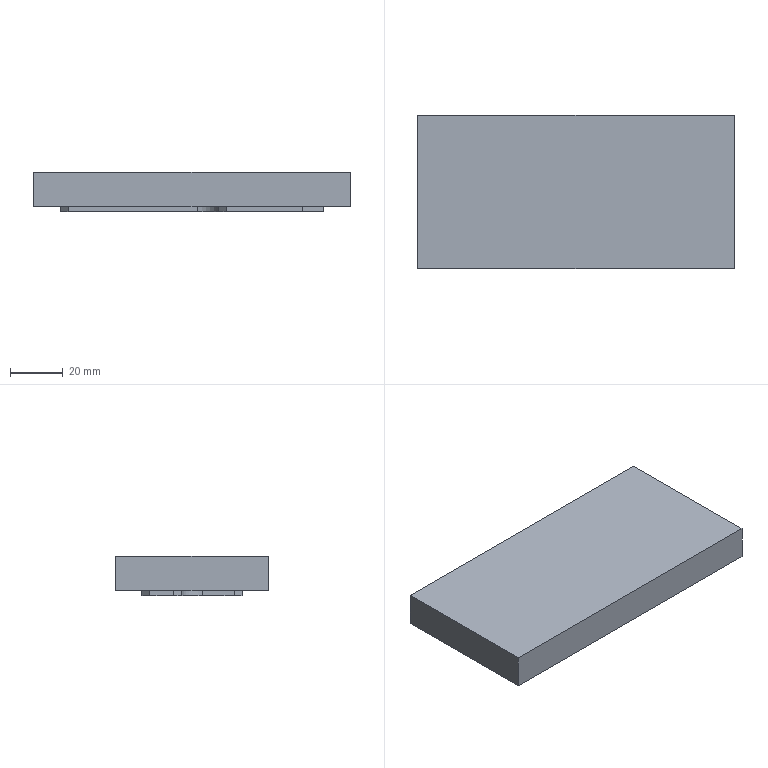NC program | NX | posted with a generic post | part box 120 x 58 x 15 mm
Whole program, first 1497 of 1693 lines:
N10 G17 G21 G94 G90
(DRILLING_COPY_1_COPY_1 , TOOL : D6A45)
N12 T01 M6
N14 G54
N16 G17 G0 G90 X-50. Y19. S5000 M3
N18 G43 Z30. H1
N20 G94 G81 G98 Z-7. F100. R3.
N22 Y-19.
N24 X-10.
N26 X50. Y4.
N28 Y19.
N30 G80
N32 G0 X50. Y19. Z30.
N34 M5
(ADAPTIVE_MILLING_COPY_COPY , TOOL : D10)
N36 T04 M6
N38 G54
N40 G17 G0 G90 X-33.307 Y3.864 S9500 M3
N42 G43 Z30. H4
N44 Z1.
N46 G94 G3 X-33.307 Y3.864 Z0.605 I2.307 J-3.864 F1000.
N48 X-33.307 Y3.864 Z0.21 I2.307 J-3.864
N50 X-33.307 Y3.864 Z-0.184 I2.307 J-3.864
N52 X-33.307 Y3.864 Z-0.579 I2.307 J-3.864
N54 X-33.307 Y3.864 Z-0.974 I2.307 J-3.864
N56 X-33.307 Y3.864 Z-1.369 I2.307 J-3.864
N58 X-33.307 Y3.864 Z-1.764 I2.307 J-3.864
N60 X-33.307 Y3.864 Z-2.158 I2.307 J-3.864
N62 X-33.307 Y3.864 Z-2.553 I2.307 J-3.864
N64 X-33.307 Y3.864 Z-2.948 I2.307 J-3.864
N66 X-33.307 Y3.864 Z-3.343 I2.307 J-3.864
N68 X-33.307 Y3.864 Z-3.738 I2.307 J-3.864
N70 X-26.5 Y0. Z-4. R-4.5
N72 X-27.321 Y-2.606 R-4.501 F3500.
N74 X-31.993 Y4.872 R4.672
N76 X-27.195 Y-3.238 R-4.977
N78 X-32.967 Y5.095 R5.193
N80 X-27.316 Y-4.074 R-5.474
N82 X-33.416 Y5.474 R5.72
N84 X-27.193 Y-4.665 R-5.999
N86 X-33.947 Y5.816 R6.26
N88 X-27.332 Y-5.436 R-6.537
N90 X-33.901 Y6.457 R6.811
N92 X-27.132 Y-5.982 R-7.099
N94 X-34.273 Y6.921 R7.384
N96 X-26.849 Y-6.497 R-7.681
N98 X-33.634 Y7.816 R7.97
N100 X-27.172 Y-7.372 R-8.275
N102 X-33.024 Y8.623 R8.576
N104 X-27.831 Y-8.335 R-8.887
N106 X-33.764 Y9.077 R9.202
N108 X-28.016 Y-9.079 R-9.522
N110 X-33.407 Y9.838 R9.841
N112 X-28.932 Y-9.985 R10.163
N114 X-20.76 Y2.399 R10.491
N116 X-33.21 Y10.557 R10.491
N118 X-29.265 Y-10.719 R10.822
N120 X-31.793 Y11.421 R11.153
N122 X-30.345 Y-11.51 R11.488
N124 X-30.043 Y12.078 R11.823
N126 X-33.673 Y-11.905 R12.157
N128 X-26.097 Y11.78 R12.486
N130 X-40.711 Y-8.472 R12.809
N132 X-18.13 Y3.189 R13.104
N134 X-42.594 Y7.072 R13.371
N136 X-23.665 Y-11.565 R13.652
N138 X-17.557 Y-3.333 R13.835
N140 X-27.736 Y13.85 R13.93
N142 X-33.859 Y13.803 R110.176
N144 X-42.857 Y8.046 R13.095
N146 X-44.85 Y3.627 R13.811
N148 X-44.816 Y-2.872 R180.518
N150 X-40.634 Y-10.629 R12.663
N152 X-34.758 Y-13.85 R14.1
N154 X-27.885 Y-13.817 R214.896
N156 X-20.139 Y-9.608 R12.747
N158 X-25.218 Y13.803 R14.699
N160 G1 X-25.34 Y13.833
N162 X-25.46 Y13.85
N164 X-33.111
N166 G3 X-36.105 Y13.756 R18.982
N168 X-42.293 Y9.973 R11.644
N170 X-44.827 Y5.986 R13.802
N172 G1 X-44.85 Y5.851
N174 Y3.601
N176 G3 X-43.97 Y2.523 R1.106
N178 X-42.879 Y2.922 Z-3.939 R1.126
N180 G1 X-42.349 Y3.492 Z-3.9
N182 X-35.048 Y11.337
N184 X-34.675 Y11.733 Z-3.927
N186 X-34.318 Y12.144 Z-3.954
N188 G3 X-34.169 Y13.017 Z-4. R1.127
N190 X-35.236 Y13.85 R1.107
N192 X-37.968 Y13.659 R9.801
N194 X-43.318 Y9.915 R11.322
N196 X-44.79 Y7.749 R12.95
N198 G1 X-44.824 Y7.629
N200 X-44.847 Y7.506
N202 X-44.85 Y7.481
N204 Y5.731
N206 G3 X-44.006 Y4.661 R1.106
N208 X-42.903 Y5.023 Z-3.939 R1.126
N210 G1 X-42.352 Y5.574 Z-3.9
N212 X-36.591 Y11.338
N214 X-35.855 Y12.092 Z-3.953
N216 G3 X-35.662 Y12.988 Z-4. R1.117
N218 X-36.736 Y13.85 R1.106
N220 X-39.216 Y13.661 R8.157
N222 X-44.182 Y10.014 R10.668
N224 X-44.85 Y8.814 R2.611
N226 G1 Y7.439
N228 G3 X-44.034 Y6.377 R1.108
N230 X-42.925 Y6.706 Z-3.939 R1.127
N232 G1 X-42.354 Y7.243 Z-3.9
N234 X-38.004 Y11.339
N236 X-37.249 Y12.066 Z-3.952
N238 G3 X-37.031 Y12.962 Z-4. R1.117
N240 X-38.111 Y13.85 R1.106
N242 X-42.657 Y12.45 R6.345
N244 X-44.744 Y10.321 R8.188
N246 G1 X-44.791 Y10.205
N248 X-44.825 Y10.084
N250 X-44.847 Y9.961
N252 X-44.85 Y9.939
N254 Y8.814
N256 G3 X-43.027 Y7.985 R1.101
N258 G1 X-38.513 Y11.921
N260 G3 X-39.236 Y13.85 R1.101
N262 X-43.835 Y12.283 R6.045
N264 X-44.826 Y11.026 R2.746
N266 G1 X-44.847 Y10.903
N268 X-44.85 Y10.884
N270 Y9.884
N272 G3 X-43.04 Y9.044 R1.101
N274 G1 X-39.65 Y11.91
N276 G3 X-40.361 Y13.85 R1.101
N278 X-44.63 Y12.219 R5.115
N280 X-44.85 Y11.641 R1.915
N282 G1 Y10.766
N284 G3 X-43.047 Y9.92 R1.101
N286 G1 X-40.658 Y11.904
N288 G3 X-41.361 Y13.85 R1.101
N290 X-43.793 Y13.447 R4.668
N292 X-44.85 Y12.222 R1.69
N294 G1 Y11.597
N296 G3 X-43.047 Y10.75 R1.101
N298 G1 X-41.658 Y11.904
N300 G3 X-42.361 Y13.85 R1.101
N302 X-44.294 Y13.501 R3.317
N304 X-44.85 Y12.12 R1.381
N306 X-42.978 Y11.337 R1.101
N308 G1 X-42.595 Y11.71
N310 X-42.225 Y12.097
N312 G3 X-43.111 Y13.85 R1.101
N314 X-44.303 Y13.691 R2.409
N316 X-44.85 Y12.586 R1.196
N318 X-44.144 Y11.63 R1.007
N320 G1 X-43.82 Y11.584 Z-3.984
N322 X-43.493 Y11.586 Z-3.967
N324 G2 X-42.78 Y11.481 Z-3.931 R1.494
N326 X-42.345 Y11.06 Z-3.9 R1.046
N328 G1 X-42.259 Y10.829
N330 X-42.225 Y10.586
N332 Y-0.373
N334 X-42.251 Y-0.583
N336 X-42.313 Y-0.784
N338 G2 X-43.314 Y-1.373 Z-3.962 R1.021
N340 G1 X-43.696 Y-1.369 Z-3.981
N342 X-44.076 Y-1.399 Z-4.
N344 G3 X-44.85 Y-2.373 R1.007
N346 X-44.745 Y-5.241 R16.119
N348 X-40.899 Y-11.393 R11.721
N350 X-37.127 Y-13.81 R14.667
N352 X-34.665 Y-13.85 R19.007
N354 X-33.592 Y-12.991 R1.106
N356 X-33.983 Y-11.882 Z-3.938 R1.125
N358 G1 X-34.539 Y-11.362 Z-3.9
N360 X-42.314 Y-4.086
N362 X-42.718 Y-3.703 Z-3.928
N364 X-43.137 Y-3.335 Z-3.956
N366 G3 X-43.983 Y-3.173 Z-4. R1.128
N368 X-44.85 Y-4.248 R1.106
N370 X-44.703 Y-6.86 R10.61
N372 X-41.125 Y-12.174 R10.997
N374 X-38.766 Y-13.801 R11.451
N376 X-36.896 Y-13.85 R10.312
N378 X-35.83 Y-13.021 R1.107
N380 X-36.185 Y-11.906 Z-3.938 R1.125
N382 G1 X-36.727 Y-11.362 Z-3.9
N384 X-42.312 Y-5.758
N386 X-42.702 Y-5.362 Z-3.928
N388 X-43.106 Y-4.981 Z-3.956
N390 G3 X-43.95 Y-4.792 Z-4. R1.127
N392 X-44.85 Y-5.873 R1.106
N394 X-44.551 Y-8.586 R7.107
N396 X-40.201 Y-13.761 R10.978
N398 G1 X-40.083 Y-13.803
N400 X-39.962 Y-13.833
N402 X-39.841 Y-13.85
N404 X-38.466
N406 G3 X-37.406 Y-13.045 R1.108
N408 X-37.73 Y-11.926 Z-3.939 R1.126
N410 G1 X-38.261 Y-11.362 Z-3.9
N412 X-42.311 Y-7.048
N414 X-42.688 Y-6.642 Z-3.928
N416 X-43.08 Y-6.251 Z-3.956
N418 G3 X-43.92 Y-6.036 Z-4. R1.127
N420 X-44.85 Y-7.123 R1.106
N422 X-43.455 Y-11.67 R6.326
N424 X-41.329 Y-13.757 R7.747
N426 G1 X-41.212 Y-13.801
N428 X-41.09 Y-13.832
N430 X-40.967 Y-13.85
N432 X-39.717
N434 G3 X-38.897 Y-12.016 R1.101
N436 G1 X-42.931 Y-7.514
N438 G3 X-44.85 Y-8.248 R1.101
N440 X-43.289 Y-12.85 R6.048
N442 X-42.028 Y-13.831 R2.605
N444 G1 X-41.904 Y-13.85
N446 X-40.904
N448 G3 X-40.063 Y-12.041 R1.101
N450 G1 X-42.909 Y-8.664
N452 G3 X-44.85 Y-9.373 R1.101
N454 X-43.221 Y-13.642 R5.114
N456 X-42.65 Y-13.85 R1.967
N458 G1 X-41.9
N460 G3 X-41.032 Y-12.074 R1.101
N462 G1 X-42.882 Y-9.697
N464 G3 X-44.85 Y-10.373 R1.101
N466 X-44.505 Y-12.694 R4.776
N468 X-43.405 Y-13.819 R1.88
N470 G1 X-43.282 Y-13.844
N472 X-43.236 Y-13.85
N474 X-42.611
N476 G3 X-41.764 Y-12.049 R1.101
N478 G1 X-42.902 Y-10.672
N480 G3 X-44.85 Y-11.373 R1.101
N482 X-44.563 Y-13.199 R3.434
N484 X-43.127 Y-13.85 R1.368
N486 X-42.347 Y-11.975 R1.101
N488 G1 X-42.717 Y-11.598
N490 X-43.101 Y-11.235
N492 G3 X-44.85 Y-12.123 R1.101
N494 X-44.691 Y-13.303 R2.38
N496 X-43.586 Y-13.85 R1.196
N498 X-42.631 Y-13.148 R1.007
N500 G1 X-42.584 Y-12.822 Z-3.983
N502 X-42.586 Y-12.493 Z-3.967
N504 G2 X-42.482 Y-11.781 Z-3.931 R1.497
N506 X-42.064 Y-11.347 Z-3.9 R1.046
N508 G1 X-41.831 Y-11.259
N510 X-41.586 Y-11.225
N512 X-30.383
N514 X-30.157 Y-11.255
N516 X-29.941 Y-11.328
N518 G2 X-29.383 Y-12.314 Z-3.96 R1.021
N520 G1 X-29.386 Y-12.68 Z-3.978
N522 X-29.362 Y-13.045 Z-3.997
N524 X-29.349 Y-13.109 Z-4.
N526 G3 X-28.383 Y-13.85 R1.007
N528 X-25.516 Y-13.735 R15.118
N530 X-19.291 Y-9.778 R11.855
N532 X-23.454 Y13.773 R15.419
N534 G1 X-23.573 Y13.812
N536 X-23.695 Y13.839
N538 X-23.774 Y13.85
N540 X-25.524
N542 G3 X-26.46 Y13.329 R1.113
N544 X-26.631 Y12.601 Z-3.962 R1.335
N546 G1 X-26.678 Y11.36 Z-3.9
N548 X-27.555 Y-11.34
N550 X-27.588 Y-12.102 Z-3.938
N552 X-27.602 Y-12.865 Z-3.976
N554 X-27.549 Y-13.095 Z-3.988
N556 X-27.455 Y-13.311 Z-4.
N558 G3 X-26.508 Y-13.85 R1.112
N560 X-23.897 Y-13.689 R10.181
N562 X-18.757 Y-10.284 R11.009
N564 X-15.05 Y-2.731 R15.824
N566 X-14.788 Y0.587 R39.404
N568 X-21.874 Y13.695 R16.044
N570 G1 X-22.352 Y13.85
N572 X-23.852
N574 G3 X-24.787 Y13.328 R1.112
N576 X-24.959 Y12.608 Z-3.963 R1.342
N578 G1 X-25.016 Y11.36 Z-3.9
N580 X-26.046 Y-11.34
N582 X-26.084 Y-12.099 Z-3.938
N584 X-26.103 Y-12.86 Z-3.976
N586 X-26.05 Y-13.092 Z-3.988
N588 X-25.955 Y-13.311 Z-4.
N590 G3 X-25.008 Y-13.85 R1.112
N592 X-22.409 Y-13.619 R7.77
N594 X-17.484 Y-9.909 R10.969
N596 X-15.159 Y-5.795 R13.627
N598 G2 X-15.04 Y-2.608 R29.836
N600 G3 X-16.035 Y-1.427 R1.104
N602 X-17.081 Y-1.949 Z-3.939 R1.125
N604 G1 X-17.536 Y-2.57 Z-3.9
N606 X-23.962 Y-11.337
N608 X-24.295 Y-11.787 Z-3.928
N610 X-24.613 Y-12.249 Z-3.956
N612 G3 X-24.675 Y-13.102 Z-4. R1.128
N614 X-23.633 Y-13.85 R1.108
N616 X-19.193 Y-12.512 R6.268
N618 X-15.208 Y-7.771 R13.615
N620 G1 X-15.174 Y-7.651
N622 X-15.153 Y-7.528
N624 X-15.15 Y-7.509
N626 Y-5.634
N628 G3 X-16.037 Y-4.555 R1.106
N630 X-17.138 Y-4.979 Z-3.938 R1.124
N632 G1 X-17.638 Y-5.547 Z-3.9
N634 X-22.73 Y-11.336
N636 X-23.094 Y-11.745 Z-3.927
N638 X-23.442 Y-12.169 Z-3.955
N640 G3 X-23.57 Y-13.038 Z-4. R1.127
N642 X-22.508 Y-13.85 R1.108
N644 X-18.101 Y-12.438 R6.033
N646 X-15.213 Y-9.193 R10.626
N648 G1 X-15.178 Y-9.073
N650 X-15.155 Y-8.95
N652 X-15.15 Y-8.917
N654 Y-7.417
N656 G3 X-15.996 Y-6.346 R1.106
N658 X-17.109 Y-6.723 Z-3.938 R1.125
N660 G1 X-17.638 Y-7.273 Z-3.9
N662 X-21.551 Y-11.338
N664 X-22.276 Y-12.108 Z-3.953
N666 G3 X-22.454 Y-13.003 Z-4. R1.118
N668 X-21.383 Y-13.85 R1.106
N670 X-17.312 Y-12.571 R5.676
N672 X-15.244 Y-10.424 R7.97
N674 G1 X-15.201 Y-10.307
N676 X-15.169 Y-10.186
N678 X-15.15 Y-10.062
N680 Y-8.812
N682 G3 X-17.009 Y-8.016 R1.101
N684 G1 X-21.142 Y-11.954
N686 G3 X-20.383 Y-13.85 R1.101
N688 X-16.235 Y-12.452 R5.53
N690 X-15.197 Y-11.227 R3.137
N692 X-15.15 Y-9.983 R6.866
N694 X-16.978 Y-9.159 R1.101
N696 G1 X-20.111 Y-11.925
N698 G3 X-19.383 Y-13.85 R1.101
N700 X-15.352 Y-12.285 R4.777
N702 X-15.15 Y-11.727 R2.132
N704 G1 Y-10.977
N706 G3 X-16.953 Y-10.131 R1.101
N708 G1 X-19.086 Y-11.904
N710 G3 X-18.383 Y-13.85 R1.101
N712 X-15.765 Y-13.235 R4.009
N714 X-15.15 Y-12.292 R1.335
N716 G1 Y-11.667
N718 G3 X-16.968 Y-10.833 R1.101
N720 G1 X-18.226 Y-11.916
N722 G3 X-17.508 Y-13.85 R1.101
N724 X-15.693 Y-13.532 R3.15
N726 X-15.15 Y-12.289 R1.253
N728 X-16.989 Y-11.474 R1.101
N730 G1 X-17.309 Y-11.763
N732 X-17.618 Y-12.064
N734 G3 X-16.758 Y-13.85 R1.101
N736 X-15.477 Y-13.523 R1.658
N738 X-15.15 Y-12.586 R1.332
N740 G1 X-15.148 Y-3.979
N742 X-14.978 Y-1.902
N744 G3 X-14.3 Y1.378 R20.921
N746 X-16.509 Y9.206 R14.048
N748 X-20.607 Y13.698 R14.647
N750 G1 X-21.081 Y13.85
N752 X-22.456
N754 G3 X-23.458 Y13.204 R1.111
N756 X-23.37 Y12.13 Z-3.944 R1.134
N758 G1 X-22.943 Y11.364 Z-3.9
N760 X-16.958 Y0.609
N762 X-16.437 Y-0.304 Z-3.953
N764 G3 X-15.625 Y-0.735 Z-4. R1.117
N766 X-14.516 Y0.023 R1.107
N768 X-13.994 Y4.855 R7.184
N770 X-19.239 Y13.574 R15.178
N772 X-19.907 Y13.85 R1.6
N774 G1 X-21.157
N776 G3 X-22.156 Y13.212 R1.111
N778 X-22.081 Y12.145 Z-3.944 R1.135
N780 G1 X-21.664 Y11.364 Z-3.9
N782 X-16.527 Y1.74
N784 X-16.272 Y1.254 Z-3.928
N786 X-15.997 Y0.778 Z-3.955
N788 G3 X-15.231 Y0.352 Z-4. R1.127
N790 X-14.108 Y1.026 R1.108
N792 X-13.356 Y3.755 R6.821
N794 X-15.217 Y10.03 R12.31
N796 X-18.244 Y13.649 R11.823
N798 X-18.8 Y13.85 R2.156
N800 G1 X-19.925
N802 G3 X-20.918 Y13.222 R1.111
N804 X-20.862 Y12.165 Z-3.945 R1.136
N806 G1 X-20.457 Y11.364 Z-3.9
N808 X-16.109 Y2.756
N810 X-15.865 Y2.264 Z-3.928
N812 X-15.601 Y1.782 Z-3.955
N814 G3 X-14.846 Y1.339 Z-4. R1.127
N816 X-13.733 Y1.931 R1.108
N818 X-12.931 Y5.586 R5.053
N820 X-16.936 Y13.447 R13.117
N822 X-17.75 Y13.85 R1.599
N824 G1 X-18.875
N826 G3 X-19.863 Y13.233 R1.111
N828 X-19.79 Y12.112 Z-3.942 R1.2
N830 G1 X-19.435 Y11.363 Z-3.9
N832 X-15.712 Y3.511
N834 X-15.472 Y2.997 Z-3.928
N836 X-15.214 Y2.492 Z-3.957
N838 G3 X-14.508 Y2.032 Z-4. R1.128
N840 X-13.368 Y2.538 R1.108
N842 X-12.475 Y6.453 R5.127
N844 X-15.893 Y13.392 R12.064
N846 X-16.763 Y13.85 R1.586
N848 G1 X-17.763
N850 G3 X-18.746 Y13.244 R1.112
N852 X-18.695 Y12.135 Z-3.942 R1.207
N854 G1 X-18.355 Y11.363 Z-3.9
N856 X-15.239 Y4.287
N858 X-15.015 Y3.771 Z-3.928
N860 X-14.773 Y3.262 Z-3.956
N862 G3 X-14.071 Y2.782 Z-4. R1.128
N864 X-12.911 Y3.285 R1.108
N866 X-11.985 Y7.003 R4.894
N868 X-15.018 Y13.438 R10.74
N870 X-15.828 Y13.85 R1.482
N872 G1 X-16.828
N874 G3 X-17.805 Y13.255 R1.112
N876 X-17.774 Y12.157 Z-3.943 R1.214
N878 G1 X-17.449 Y11.363 Z-3.9
N880 X-14.832 Y4.955
N882 X-14.62 Y4.427 Z-3.929
N884 X-14.389 Y3.906 Z-3.957
N886 G3 X-13.714 Y3.408 Z-4. R1.129
N888 X-12.611 Y3.761 R1.112
N890 X-11.462 Y6.957 R4.134
N892 X-14.102 Y13.404 R9.713
N894 X-14.957 Y13.85 R1.48
N896 G1 X-15.832
N898 G3 X-16.801 Y13.27 R1.112
N900 X-16.802 Y12.195 Z-3.944 R1.226
N902 G1 X-16.504 Y11.362 Z-3.9
N904 X-14.411 Y5.512
N906 X-14.219 Y4.966 Z-3.929
N908 X-14.009 Y4.427 Z-3.958
N910 G3 X-13.376 Y3.903 Z-4. R1.129
N912 X-12.206 Y4.236 R1.108
N914 X-10.969 Y7.527 R4.225
N916 X-13.303 Y13.435 R8.688
N918 X-14.111 Y13.85 R1.436
N920 G1 X-14.986
N922 G3 X-15.952 Y13.276 R1.112
N924 X-15.997 Y12.305 Z-3.95 R1.149
N926 G1 X-15.679 Y11.362 Z-3.9
N928 X-13.91 Y6.101
N930 X-13.73 Y5.555 Z-3.929
N932 X-13.531 Y5.014 Z-3.958
N934 G3 X-12.902 Y4.477 Z-4. R1.129
N936 X-11.718 Y4.807 R1.108
N938 X-10.474 Y8.075 R4.231
N940 X-12.518 Y13.44 R7.864
N942 X-13.313 Y13.85 R1.382
N944 G1 X-14.188
N946 G3 X-15.239 Y12.423 R1.103
N948 G1 X-13.154 Y5.718
N950 G3 X-11.326 Y5.267 R1.102
N952 X-10.001 Y7.944 R3.565
N954 X-11.809 Y13.484 R7.158
N956 X-12.566 Y13.85 R1.352
N958 G1 X-13.316
N960 G3 X-14.381 Y12.478 R1.103
N962 G1 X-12.762 Y6.133
N964 G3 X-10.982 Y5.569 R1.102
N966 X-9.486 Y8.466 R3.71
N968 X-11.063 Y13.45 R6.561
N970 X-11.841 Y13.85 R1.336
N972 G1 X-12.591
N974 G3 X-13.663 Y12.503 R1.103
N976 G1 X-12.293 Y6.564
N978 G3 X-10.506 Y5.975 R1.102
N980 X-8.973 Y8.982 R3.768
N982 X-10.426 Y13.496 R5.956
N984 X-11.159 Y13.85 R1.32
N986 G1 X-11.909
N988 G3 X-12.985 Y12.524 R1.103
N990 G1 X-11.822 Y6.991
N992 G3 X-10.031 Y6.381 R1.102
N994 X-8.478 Y9.307 R3.646
N996 X-9.769 Y13.489 R5.502
N998 X-10.509 Y13.85 R1.296
N1000 G1 X-11.259
N1002 G3 X-12.339 Y12.542 R1.103
N1004 G1 X-11.349 Y7.391
N1006 G3 X-9.694 Y6.66 R1.102
N1008 X-8.064 Y9.044 R3.141
N1010 X-9.071 Y13.408 R5.268
N1012 X-9.884 Y13.85 R1.281
N1014 G1 X-10.634
N1016 G3 X-11.72 Y12.574 R1.103
N1018 G1 X-10.928 Y7.684
N1020 G3 X-9.267 Y6.922 R1.102
N1022 X-7.537 Y9.517 R3.279
N1024 X-8.566 Y13.5 R4.818
N1026 X-9.289 Y13.85 R1.294
N1028 G1 X-9.914
N1030 G3 X-11.008 Y12.632 R1.103
N1032 G1 X-10.51 Y8.003
N1034 G3 X-8.841 Y7.183 R1.102
N1036 X-7.04 Y9.865 R3.3
N1038 X-7.994 Y13.499 R4.491
N1040 X-8.72 Y13.85 R1.295
N1042 G1 X-9.345
N1044 G3 X-10.438 Y12.633 R1.103
N1046 G1 X-9.977 Y8.33
N1048 G3 X-8.308 Y7.509 R1.102
N1050 X-6.581 Y10.028 R3.15
N1052 X-7.488 Y13.54 R4.186
N1054 X-8.796 Y13.85 R1.709
N1056 X-9.889 Y12.629 R1.103
N1058 G1 X-9.446 Y8.628
N1060 G3 X-7.931 Y7.733 R1.103
N1062 X-6.223 Y9.739 R2.737
N1064 X-6.938 Y13.514 R4.066
N1066 X-7.645 Y13.85 R1.319
N1068 G1 X-8.27
N1070 G3 X-9.367 Y12.675 R1.104
N1072 G1 X-9.103 Y8.817
N1074 G3 X-7.585 Y7.876 R1.102
N1076 X-5.73 Y10.053 R2.81
N1078 X-6.487 Y13.571 R3.767
N1080 X-7.768 Y13.85 R1.769
N1082 X-8.866 Y12.683 R1.104
N1084 G1 X-8.642 Y9.017
N1086 G3 X-7.123 Y8.068 R1.102
N1088 X-5.272 Y10.245 R2.796
N1090 X-5.961 Y13.541 R3.641
N1092 X-7.267 Y13.85 R1.711
N1094 X-8.365 Y12.692 R1.104
N1096 G1 X-8.18 Y9.217
N1098 G3 X-6.661 Y8.259 R1.102
N1100 X-4.821 Y10.442 R2.762
N1102 X-5.545 Y13.596 R3.361
N1104 X-6.664 Y13.85 R1.592
N1106 X-7.764 Y12.735 R1.104
N1108 G1 X-7.72 Y9.452
N1110 G3 X-6.199 Y8.45 R1.102
N1112 X-4.492 Y10.209 R2.484
N1114 X-5. Y13.52 R3.417
N1116 X-6.201 Y13.85 R1.501
N1118 X-7.301 Y12.777 R1.104
N1120 G1 X-7.379 Y9.613
N1122 G3 X-6.023 Y8.516 R1.103
N1124 X-4.088 Y10.26 R2.427
N1126 X-4.59 Y13.558 R3.265
N1128 X-5.766 Y13.85 R1.564
N1130 X-6.866 Y12.76 R1.104
N1132 G1 X-6.894 Y9.712
N1134 G3 X-5.537 Y8.633 R1.103
N1136 X-3.645 Y10.427 R2.446
N1138 X-4.098 Y13.508 R3.225
N1140 X-5.312 Y13.85 R1.492
N1142 X-6.411 Y12.794 R1.104
N1144 G1 X-6.528 Y9.834
N1146 G3 X-5.172 Y8.72 R1.103
N1148 X-3.206 Y10.594 R2.471
N1150 X-3.699 Y13.544 R3.068
N1152 X-4.878 Y13.85 R1.527
N1154 X-5.975 Y12.821 R1.104
N1156 G1 X-6.162 Y9.949
N1158 G3 X-4.808 Y8.808 R1.103
N1160 X-2.769 Y10.759 R2.494
N1162 X-3.312 Y13.578 R2.925
N1164 X-4.456 Y13.85 R1.574
N1166 X-5.555 Y12.799 R1.104
N1168 G1 X-5.677 Y10.043
N1170 G3 X-4.321 Y8.925 R1.103
N1172 X-2.431 Y10.627 R2.349
N1174 X-2.882 Y13.57 R2.899
N1176 X-4.04 Y13.85 R1.569
N1178 X-5.139 Y12.776 R1.104
N1180 G1 X-5.202 Y10.114
N1182 G3 X-4.015 Y8.991 R1.103
N1184 X-2.137 Y10.423 R2.153
N1186 X-2.405 Y13.504 R2.993
N1188 X-3.624 Y13.85 R1.49
N1190 X-4.72 Y12.845 R1.106
N1192 G1 X-4.948 Y10.203
N1194 G3 X-3.766 Y9.011 R1.103
N1196 X-1.751 Y10.443 R2.199
N1198 X-2.016 Y13.517 R2.92
N1200 X-3.22 Y13.85 R1.499
N1202 X-4.315 Y12.858 R1.106
N1204 G1 X-4.573 Y10.245
N1206 G3 X-3.392 Y9.04 R1.103
N1208 X-1.318 Y10.576 R2.244
N1210 X-1.63 Y13.53 R2.841
N1212 X-2.821 Y13.85 R1.511
N1214 X-3.914 Y12.87 R1.106
N1216 G1 X-4.198 Y10.287
N1218 G3 X-3.019 Y9.07 R1.103
N1220 X-0.933 Y10.591 R2.239
N1222 X-1.241 Y13.541 R2.796
N1224 X-2.422 Y13.85 R1.524
N1226 X-3.514 Y12.882 R1.106
N1228 G1 X-3.823 Y10.328
N1230 G3 X-2.645 Y9.099 R1.103
N1232 X-0.547 Y10.606 R2.253
N1234 X-0.857 Y13.552 R2.765
N1236 X-2.032 Y13.85 R1.543
N1238 X-3.123 Y12.891 R1.106
N1240 G1 X-3.448 Y10.366
N1242 G3 X-2.271 Y9.129 R1.103
N1244 X-0.2 Y10.543 R2.207
N1246 X-0.415 Y13.503 R2.82
N1248 X-1.634 Y13.85 R1.489
N1250 X-2.723 Y12.901 R1.106
N1252 G1 X-3.069 Y10.401
N1254 G3 X-1.979 Y9.15 R1.103
N1256 X0.123 Y10.434 R2.14
N1258 X-0.025 Y13.504 R2.822
N1260 X-1.243 Y13.85 R1.49
N1262 X-2.331 Y12.907 R1.106
N1264 G1 X-2.693 Y10.407
N1266 G3 X-1.604 Y9.15 R1.103
N1268 X0.502 Y10.433 R2.164
N1270 X0.363 Y13.503 R2.808
N1272 X-0.857 Y13.85 R1.489
N1274 X-1.945 Y12.912 R1.106
N1276 G1 X-2.317 Y10.412
N1278 G3 X-1.229 Y9.15 R1.103
N1280 X0.938 Y10.541 R2.204
N1282 X0.751 Y13.499 R2.779
N1284 X-0.474 Y13.85 R1.487
N1286 X-1.561 Y12.915 R1.106
N1288 G1 X-1.942 Y10.415
N1290 G3 X-0.854 Y9.15 R1.103
N1292 X1.261 Y10.424 R2.184
N1294 X1.14 Y13.494 R2.809
N1296 X-0.09 Y13.85 R1.484
N1298 X-1.177 Y12.919 R1.106
N1300 G1 X-1.566 Y10.419
N1302 G3 X-0.479 Y9.15 R1.103
N1304 X1.698 Y10.53 R2.22
N1306 X1.53 Y13.49 R2.796
N1308 X0.295 Y13.85 R1.483
N1310 X-0.791 Y12.923 R1.106
N1312 G1 X-1.19 Y10.423
N1314 G3 X-0.104 Y9.15 R1.103
N1316 X2.076 Y10.524 R2.218
N1318 X1.918 Y13.484 R2.791
N1320 X0.676 Y13.85 R1.481
N1322 X-0.41 Y12.926 R1.106
N1324 G1 X-0.815 Y10.426
N1326 G3 X0.271 Y9.15 R1.103
N1328 X2.457 Y10.518 R2.228
N1330 X2.309 Y13.478 R2.786
N1332 X1.059 Y13.85 R1.479
N1334 X-0.027 Y12.929 R1.106
N1336 G1 X-0.439 Y10.429
N1338 G3 X0.646 Y9.15 R1.103
N1340 X2.836 Y10.509 R2.218
N1342 X2.7 Y13.473 R2.811
N1344 X1.443 Y13.85 R1.478
N1346 X0.358 Y12.933 R1.106
N1348 G1 X-0.064 Y10.433
N1350 G3 X1.021 Y9.15 R1.103
N1352 X3.215 Y10.503 R2.22
N1354 X3.091 Y13.467 R2.815
N1356 X1.828 Y13.85 R1.474
N1358 X0.744 Y12.937 R1.106
N1360 G1 X0.312 Y10.437
N1362 G3 X1.396 Y9.15 R1.103
N1364 X3.598 Y10.494 R2.237
N1366 X3.479 Y13.459 R2.81
N1368 X2.22 Y13.85 R1.454
N1370 X1.137 Y12.944 R1.106
N1372 G1 X0.688 Y10.444
N1374 G3 X1.771 Y9.15 R1.103
N1376 X3.976 Y10.486 R2.224
N1378 X3.871 Y13.452 R2.822
N1380 X2.607 Y13.85 R1.447
N1382 X1.525 Y12.949 R1.106
N1384 G1 X1.064 Y10.449
N1386 G3 X2.146 Y9.15 R1.103
N1388 X4.356 Y10.478 R2.223
N1390 X4.177 Y13.538 R2.743
N1392 X2.993 Y13.85 R1.519
N1394 X1.912 Y12.954 R1.106
N1396 G1 X1.44 Y10.454
N1398 G3 X2.521 Y9.15 R1.103
N1400 X4.736 Y10.47 R2.223
N1402 X4.568 Y13.53 R2.753
N1404 X3.377 Y13.85 R1.511
N1406 X2.288 Y12.905 R1.106
N1408 G1 X1.932 Y10.405
N1410 G3 X3.021 Y9.15 R1.103
N1412 X5.115 Y10.461 R2.188
N1414 X4.959 Y13.523 R2.758
N1416 X3.761 Y13.85 R1.504
N1418 X2.673 Y12.909 R1.106
N1420 G1 X2.307 Y10.409
N1422 G3 X3.396 Y9.15 R1.103
N1424 X5.498 Y10.452 R2.211
N1426 X5.354 Y13.518 R2.781
N1428 X4.151 Y13.85 R1.499
N1430 X3.063 Y12.915 R1.106
N1432 G1 X2.683 Y10.415
N1434 G3 X3.771 Y9.15 R1.103
N1436 X5.878 Y10.444 R2.203
N1438 X5.745 Y13.511 R2.776
N1440 X4.534 Y13.85 R1.494
N1442 X3.447 Y12.919 R1.106
N1444 G1 X3.059 Y10.419
N1446 G3 X4.146 Y9.15 R1.103
N1448 X6.313 Y10.546 R2.221
N1450 X6.135 Y13.503 R2.765
N1452 X4.915 Y13.85 R1.489
N1454 X3.828 Y12.921 R1.106
N1456 G1 X3.434 Y10.421
N1458 G3 X4.521 Y9.15 R1.103
N1460 X6.637 Y10.427 R2.196
N1462 X6.526 Y13.495 R2.8
N1464 X5.297 Y13.85 R1.485
N1466 X4.211 Y12.924 R1.106
N1468 G1 X3.81 Y10.424
N1470 G3 X4.896 Y9.15 R1.103
N1472 X7.075 Y10.529 R2.23
N1474 X6.913 Y13.488 R2.788
N1476 X5.676 Y13.85 R1.482
N1478 X4.59 Y12.926 R1.106
N1480 G1 X4.185 Y10.426
N1482 G3 X5.271 Y9.15 R1.103
N1484 X7.454 Y10.522 R2.226
N1486 X7.302 Y13.481 R2.778
N1488 X6.055 Y13.85 R1.48
N1490 X4.97 Y12.928 R1.106
N1492 G1 X4.56 Y10.428
N1494 G3 X5.646 Y9.15 R1.103
N1496 X7.835 Y10.515 R2.232
N1498 X7.694 Y13.477 R2.8
N1500 X6.441 Y13.85 R1.479
N1502 X5.357 Y12.932 R1.106
N1504 G1 X4.936 Y10.432
N1506 G3 X6.021 Y9.15 R1.103
N1508 X8.213 Y10.506 R2.218
N1510 X8.087 Y13.469 R2.814
N1512 X6.824 Y13.85 R1.478
N1514 X5.74 Y12.936 R1.106
N1516 G1 X5.312 Y10.436
N1518 G3 X6.396 Y9.15 R1.103
N1520 X8.597 Y10.497 R2.239
N1522 X8.476 Y13.461 R2.811
N1524 X7.216 Y13.85 R1.46
N1526 X6.133 Y12.943 R1.106
N1528 G1 X5.688 Y10.443
N1530 G3 X6.771 Y9.15 R1.103
N1532 X8.976 Y10.489 R2.235
N1534 X8.866 Y13.454 R2.818
N1536 X7.603 Y13.85 R1.45
N1538 X6.521 Y12.948 R1.106
N1540 G1 X6.064 Y10.448
N1542 G3 X7.146 Y9.15 R1.103
N1544 X9.41 Y10.594 R2.255
N1546 X9.171 Y13.54 R2.72
N1548 X7.99 Y13.85 R1.523
N1550 X6.909 Y12.953 R1.106
N1552 G1 X6.44 Y10.453
N1554 G3 X7.521 Y9.15 R1.103
N1556 X9.736 Y10.471 R2.227
N1558 X9.563 Y13.531 R2.751
N1560 X8.373 Y13.85 R1.512
N1562 X7.284 Y12.904 R1.106
N1564 G1 X6.932 Y10.404
N1566 G3 X8.021 Y9.15 R1.103
N1568 X10.115 Y10.462 R2.19
N1570 X9.954 Y13.524 R2.758
N1572 X8.757 Y13.85 R1.505
N1574 X7.669 Y12.907 R1.106
N1576 G1 X7.307 Y10.407
N1578 G3 X8.396 Y9.15 R1.103
N1580 X10.495 Y10.455 R2.198
N1582 X10.347 Y13.519 R2.772
N1584 X9.145 Y13.85 R1.501
N1586 X8.057 Y12.913 R1.106
N1588 G1 X7.683 Y10.413
N1590 G3 X8.771 Y9.15 R1.103
N1592 X10.876 Y10.446 R2.202
N1594 X10.741 Y13.512 R2.783
N1596 X9.532 Y13.85 R1.495
N1598 X8.445 Y12.918 R1.106
N1600 G1 X8.059 Y10.418
N1602 G3 X9.146 Y9.15 R1.103
N1604 X11.255 Y10.438 R2.189
N1606 X11.129 Y13.504 R2.778
N1608 X9.911 Y13.85 R1.49
N1610 X8.824 Y12.92 R1.106
N1612 G1 X8.434 Y10.42
N1614 G3 X9.521 Y9.15 R1.103
N1616 X11.636 Y10.428 R2.195
N1618 X11.521 Y13.497 R2.8
N1620 X10.294 Y13.85 R1.485
N1622 X9.207 Y12.923 R1.106
N1624 G1 X8.81 Y10.423
N1626 G3 X9.896 Y9.15 R1.103
N1628 X12.074 Y10.532 R2.235
N1630 X11.909 Y13.491 R2.787
N1632 X10.675 Y13.85 R1.483
N1634 X9.589 Y12.926 R1.106
N1636 G1 X9.185 Y10.426
N1638 G3 X10.271 Y9.15 R1.103
N1640 X12.452 Y10.524 R2.224
N1642 X12.299 Y13.484 R2.782
N1644 X11.056 Y13.85 R1.481
N1646 X9.971 Y12.928 R1.106
N1648 G1 X9.56 Y10.428
N1650 G3 X10.646 Y9.15 R1.103
N1652 X12.835 Y10.516 R2.233
N1654 X12.693 Y13.477 R2.798
N1656 X11.441 Y13.85 R1.479
N1658 X10.356 Y12.932 R1.106
N1660 G1 X9.936 Y10.432
N1662 G3 X11.021 Y9.15 R1.103
N1664 X13.212 Y10.507 R2.215
N1666 X13.084 Y13.47 R2.818
N1668 X11.823 Y13.85 R1.478
N1670 X10.739 Y12.935 R1.106
N1672 G1 X10.312 Y10.435
N1674 G3 X11.396 Y9.15 R1.103
N1676 X13.595 Y10.499 R2.235
N1678 X13.475 Y13.463 R2.808
N1680 X12.213 Y13.85 R1.464
N1682 X11.13 Y12.942 R1.106
N1684 G1 X10.688 Y10.442
N1686 G3 X11.771 Y9.15 R1.103
N1688 X13.975 Y10.491 R2.241
N1690 X13.864 Y13.456 R2.814
N1692 X12.603 Y13.85 R1.452
N1694 X11.521 Y12.948 R1.106
N1696 G1 X11.064 Y10.448
N1698 G3 X12.146 Y9.15 R1.103
N1700 X14.354 Y10.483 R2.224
N1702 X14.17 Y13.542 R2.747
N1704 X12.99 Y13.85 R1.525
N1706 X11.909 Y12.953 R1.106
N1708 G1 X11.44 Y10.453
N1710 G3 X12.521 Y9.15 R1.103
N1712 X14.733 Y10.473 R2.218
N1714 X14.561 Y13.533 R2.746
N1716 X13.373 Y13.85 R1.514
N1718 X12.284 Y12.904 R1.106
N1720 G1 X11.932 Y10.404
N1722 G3 X13.021 Y9.15 R1.103
N1724 X15.054 Y10.354 R2.161
N1726 X15.034 Y13.432 R2.849
N1728 X13.756 Y13.85 R1.431
N1730 X12.667 Y12.907 R1.106
N1732 G1 X12.307 Y10.407
N1734 G3 X13.396 Y9.15 R1.103
N1736 X15.493 Y10.457 R2.194
N1738 X15.344 Y13.52 R2.766
N1740 X14.143 Y13.85 R1.501
N1742 X13.055 Y12.912 R1.106
N1744 G1 X12.683 Y10.412
N1746 G3 X13.771 Y9.15 R1.103
N1748 X15.875 Y10.448 R2.201
N1750 X15.736 Y13.514 R2.781
N1752 X14.529 Y13.85 R1.496
N1754 X13.441 Y12.917 R1.106
N1756 G1 X13.059 Y10.417
N1758 G3 X14.146 Y9.15 R1.103
N1760 X16.254 Y10.439 R2.189
N1762 X16.126 Y13.506 R2.781
N1764 X14.91 Y13.85 R1.491
N1766 X13.823 Y12.919 R1.106
N1768 G1 X13.434 Y10.419
N1770 G3 X14.521 Y9.15 R1.103
N1772 X16.635 Y10.429 R2.192
N1774 X16.516 Y13.497 R2.796
N1776 X15.29 Y13.85 R1.486
N1778 X14.203 Y12.921 R1.106
N1780 G1 X13.809 Y10.421
N1782 G3 X14.896 Y9.15 R1.103
N1784 X17.074 Y10.533 R2.236
N1786 X16.907 Y13.491 R2.786
N1788 X15.673 Y13.85 R1.483
N1790 X14.587 Y12.925 R1.106
N1792 G1 X14.185 Y10.425
N1794 G3 X15.271 Y9.15 R1.103
N1796 X17.451 Y10.526 R2.224
N1798 X17.296 Y13.485 R2.783
N1800 X16.054 Y13.85 R1.481
N1802 X14.969 Y12.927 R1.106
N1804 G1 X14.56 Y10.427
N1806 G3 X15.646 Y9.15 R1.103
N1808 X17.833 Y10.518 R2.231
N1810 X17.688 Y13.479 R2.79
N1812 X16.438 Y13.85 R1.479
N1814 X15.353 Y12.931 R1.106
N1816 G1 X14.936 Y10.431
N1818 G3 X16.021 Y9.15 R1.103
N1820 X18.212 Y10.509 R2.221
N1822 X18.079 Y13.473 R2.822
N1824 X16.822 Y13.85 R1.478
N1826 X15.738 Y12.935 R1.106
N1828 G1 X15.312 Y10.435
N1830 G3 X16.396 Y9.15 R1.103
N1832 X18.591 Y10.502 R2.222
N1834 X18.471 Y13.466 R2.815
N1836 X17.208 Y13.85 R1.472
N1838 X16.124 Y12.939 R1.106
N1840 G1 X15.687 Y10.439
N1842 G3 X16.771 Y9.15 R1.103
N1844 X18.973 Y10.494 R2.238
N1846 X18.859 Y13.459 R2.815
N1848 X17.6 Y13.85 R1.455
N1850 X16.517 Y12.947 R1.106
N1852 G1 X16.064 Y10.447
N1854 G3 X17.146 Y9.15 R1.103
N1856 X19.352 Y10.486 R2.225
N1858 X19.166 Y13.544 R2.744
N1860 X17.987 Y13.85 R1.528
N1862 X16.906 Y12.952 R1.106
N1864 G1 X16.44 Y10.452
N1866 G3 X17.521 Y9.15 R1.103
N1868 X19.732 Y10.477 R2.224
N1870 X19.557 Y13.536 R2.741
N1872 X18.372 Y13.85 R1.518
N1874 X17.291 Y12.956 R1.106
N1876 G1 X16.815 Y10.456
N1878 G3 X17.896 Y9.15 R1.103
N1880 X20.112 Y10.469 R2.225
N1882 X19.945 Y13.529 R2.749
N1884 X18.753 Y13.85 R1.51
N1886 X17.664 Y12.905 R1.106
N1888 G1 X17.307 Y10.405
N1890 G3 X18.396 Y9.15 R1.103
N1892 X20.49 Y10.461 R2.186
N1894 X20.337 Y13.523 R2.755
N1896 X19.138 Y13.85 R1.504
N1898 X18.05 Y12.91 R1.106
N1900 G1 X17.683 Y10.41
N1902 G3 X18.771 Y9.15 R1.103
N1904 X20.874 Y10.453 R2.213
N1906 X20.73 Y13.518 R2.78
N1908 X19.527 Y13.85 R1.5
N1910 X18.439 Y12.916 R1.106
N1912 G1 X18.058 Y10.416
N1914 G3 X19.146 Y9.15 R1.103
N1916 X21.253 Y10.444 R2.204
N1918 X21.12 Y13.511 R2.778
N1920 X19.91 Y13.85 R1.494
N1922 X18.823 Y12.919 R1.106
N1924 G1 X18.434 Y10.419
N1926 G3 X19.521 Y9.15 R1.103
N1928 X21.688 Y10.546 R2.221
N1930 X21.51 Y13.503 R2.769
N1932 X20.291 Y13.85 R1.489
N1934 X19.204 Y12.922 R1.106
N1936 G1 X18.809 Y10.422
N1938 G3 X19.896 Y9.15 R1.103
N1940 X22.012 Y10.426 R2.198
N1942 X21.901 Y13.495 R2.799
N1944 X20.672 Y13.85 R1.485
N1946 X19.586 Y12.924 R1.106
N1948 G1 X19.185 Y10.424
N1950 G3 X20.271 Y9.15 R1.103
N1952 X22.449 Y10.53 R2.228
N1954 X22.289 Y13.489 R2.785
N1956 X21.052 Y13.85 R1.482
N1958 X19.967 Y12.926 R1.106
N1960 G1 X19.56 Y10.426
N1962 G3 X20.646 Y9.15 R1.103
N1964 X22.83 Y10.522 R2.229
N1966 X22.678 Y13.481 R2.777
N1968 X21.432 Y13.85 R1.48
N1970 X20.346 Y12.928 R1.106
N1972 G1 X19.935 Y10.428
N1974 G3 X21.021 Y9.15 R1.103
N1976 X23.21 Y10.514 R2.233
N1978 X23.07 Y13.476 R2.802
N1980 X21.817 Y13.85 R1.479
N1982 X20.733 Y12.933 R1.106
N1984 G1 X20.311 Y10.433
N1986 G3 X21.396 Y9.15 R1.103
N1988 X23.588 Y10.506 R2.215
N1990 X23.462 Y13.47 R2.815
N1992 X22.201 Y13.85 R1.478
N1994 X21.116 Y12.936 R1.106
N1996 G1 X20.687 Y10.436
N1998 G3 X21.771 Y9.15 R1.103
N2000 X23.971 Y10.498 R2.238
N2002 X23.851 Y13.462 R2.811
N2004 X22.591 Y13.85 R1.462
N2006 X21.508 Y12.943 R1.106
N2008 G1 X21.063 Y10.443
N2010 G3 X22.146 Y9.15 R1.103
N2012 X24.351 Y10.49 R2.239
N2014 X24.241 Y13.456 R2.815
N2016 X22.979 Y13.85 R1.451
N2018 X21.897 Y12.948 R1.106
N2020 G1 X21.439 Y10.448
N2022 G3 X22.521 Y9.15 R1.103
N2024 X24.729 Y10.482 R2.224
N2026 X24.548 Y13.541 R2.743
N2028 X23.367 Y13.85 R1.524
N2030 X22.286 Y12.954 R1.106
N2032 G1 X21.815 Y10.454
N2034 G3 X22.896 Y9.15 R1.103
N2036 X25.111 Y10.471 R2.226
N2038 X24.941 Y13.532 R2.753
N2040 X23.752 Y13.85 R1.513
N2042 X22.663 Y12.905 R1.106
N2044 G1 X22.307 Y10.405
N2046 G3 X23.396 Y9.15 R1.103
N2048 X25.49 Y10.462 R2.191
N2050 X25.332 Y13.525 R2.756
N2052 X24.136 Y13.85 R1.505
N2054 X23.047 Y12.909 R1.106
N2056 G1 X22.682 Y10.409
N2058 G3 X23.771 Y9.15 R1.103
N2060 X25.872 Y10.454 R2.206
N2062 X25.725 Y13.519 R2.781
N2064 X24.523 Y13.85 R1.501
N2066 X23.436 Y12.914 R1.106
N2068 G1 X23.058 Y10.414
N2070 G3 X24.146 Y9.15 R1.103
N2072 X26.251 Y10.445 R2.201
N2074 X26.118 Y13.512 R2.78
N2076 X24.909 Y13.85 R1.495
N2078 X23.822 Y12.919 R1.106
N2080 G1 X23.434 Y10.419
N2082 G3 X24.521 Y9.15 R1.103
N2084 X26.631 Y10.437 R2.193
N2086 X26.507 Y13.504 R2.781
N2088 X25.288 Y13.85 R1.489
N2090 X24.202 Y12.921 R1.106
N2092 G1 X23.809 Y10.421
N2094 G3 X24.896 Y9.15 R1.103
N2096 X27.012 Y10.427 R2.199
N2098 X26.898 Y13.496 R2.802
N2100 X25.67 Y13.85 R1.485
N2102 X24.584 Y12.923 R1.106
N2104 G1 X24.185 Y10.423
N2106 G3 X25.271 Y9.15 R1.103
N2108 X27.45 Y10.53 R2.231
N2110 X27.286 Y13.489 R2.785
N2112 X26.049 Y13.85 R1.482
N2114 X24.963 Y12.925 R1.106
N2116 G1 X24.56 Y10.425
N2118 G3 X25.646 Y9.15 R1.103
N2120 X27.829 Y10.522 R2.227
N2122 X27.676 Y13.482 R2.784
N2124 X26.43 Y13.85 R1.48
N2126 X25.344 Y12.927 R1.106
N2128 G1 X24.935 Y10.427
N2130 G3 X26.021 Y9.15 R1.103
N2132 X28.21 Y10.515 R2.232
N2134 X28.069 Y13.477 R2.8
N2136 X26.816 Y13.85 R1.479
N2138 X25.731 Y12.932 R1.106
N2140 G1 X25.311 Y10.432
N2142 G3 X26.396 Y9.15 R1.103
N2144 X28.587 Y10.507 R2.215
N2146 X28.46 Y13.47 R2.815
N2148 X27.198 Y13.85 R1.478
N2150 X26.114 Y12.935 R1.106
N2152 G1 X25.687 Y10.435
N2154 G3 X26.771 Y9.15 R1.103
N2156 X28.97 Y10.499 R2.235
N2158 X28.85 Y13.463 R2.809
N2160 X27.589 Y13.85 R1.464
N2162 X26.505 Y12.942 R1.106
N2164 G1 X26.063 Y10.442
N2166 G3 X27.146 Y9.15 R1.103
N2168 X29.35 Y10.491 R2.241
N2170 X29.238 Y13.456 R2.815
N2172 X27.977 Y13.85 R1.452
N2174 X26.895 Y12.947 R1.106
N2176 G1 X26.439 Y10.447
N2178 G3 X27.521 Y9.15 R1.103
N2180 X29.729 Y10.483 R2.224
N2182 X29.544 Y13.542 R2.748
N2184 X28.364 Y13.85 R1.525
N2186 X27.283 Y12.952 R1.106
N2188 G1 X26.815 Y10.452
N2190 G3 X27.896 Y9.15 R1.103
N2192 X30.108 Y10.473 R2.218
N2194 X29.936 Y13.533 R2.747
N2196 X28.748 Y13.85 R1.514
N2198 X27.659 Y12.903 R1.106
N2200 G1 X27.307 Y10.403
N2202 G3 X28.396 Y9.15 R1.103
N2204 X30.488 Y10.465 R2.188
N2206 X30.325 Y13.526 R2.748
N2208 X29.13 Y13.85 R1.506
N2210 X28.041 Y12.906 R1.106
N2212 G1 X27.682 Y10.406
N2214 G3 X28.771 Y9.15 R1.103
N2216 X30.868 Y10.457 R2.191
N2218 X30.718 Y13.52 R2.765
N2220 X29.517 Y13.85 R1.501
N2222 X28.429 Y12.912 R1.106
N2224 G1 X28.058 Y10.412
N2226 G3 X29.146 Y9.15 R1.103
N2228 X31.25 Y10.448 R2.201
N2230 X31.11 Y13.514 R2.78
N2232 X29.903 Y13.85 R1.496
N2234 X28.815 Y12.916 R1.106
N2236 G1 X28.433 Y10.416
N2238 G3 X29.521 Y9.15 R1.103
N2240 X31.628 Y10.44 R2.186
N2242 X31.499 Y13.506 R2.776
N2244 X30.284 Y13.85 R1.491
N2246 X29.197 Y12.919 R1.106
N2248 G1 X28.809 Y10.419
N2250 G3 X29.896 Y9.15 R1.103
N2252 X32.01 Y10.43 R2.193
N2254 X31.891 Y13.498 R2.793
N2256 X30.665 Y13.85 R1.486
N2258 X29.578 Y12.921 R1.106
N2260 G1 X29.184 Y10.421
N2262 G3 X30.271 Y9.15 R1.103
N2264 X32.448 Y10.533 R2.234
N2266 X32.281 Y13.492 R2.786
N2268 X31.048 Y13.85 R1.483
N2270 X29.962 Y12.925 R1.106
N2272 G1 X29.56 Y10.425
N2274 G3 X30.646 Y9.15 R1.103
N2276 X32.826 Y10.526 R2.226
N2278 X32.67 Y13.486 R2.784
N2280 X31.43 Y13.85 R1.481
N2282 X30.344 Y12.928 R1.106
N2284 G1 X29.935 Y10.428
N2286 G3 X31.021 Y9.15 R1.103
N2288 X33.208 Y10.518 R2.232
N2290 X33.062 Y13.479 R2.788
N2292 X31.812 Y13.85 R1.479
N2294 X30.727 Y12.931 R1.106
N2296 G1 X30.311 Y10.431
N2298 G3 X31.396 Y9.15 R1.103
N2300 X33.587 Y10.509 R2.225
N2302 X33.453 Y13.474 R2.822
N2304 X32.197 Y13.85 R1.478
N2306 X31.112 Y12.935 R1.106
N2308 G1 X30.686 Y10.435
N2310 G3 X31.771 Y9.15 R1.103
N2312 X33.966 Y10.502 R2.221
N2314 X33.845 Y13.467 R2.816
N2316 X32.582 Y13.85 R1.474
N2318 X31.498 Y12.939 R1.106
N2320 G1 X31.062 Y10.439
N2322 G3 X32.146 Y9.15 R1.103
N2324 X34.348 Y10.494 R2.238
N2326 X34.235 Y13.459 R2.817
N2328 X32.975 Y13.85 R1.455
N2330 X31.893 Y12.947 R1.106
N2332 G1 X31.439 Y10.447
N2334 G3 X32.521 Y9.15 R1.103
N2336 X34.727 Y10.486 R2.225
N2338 X34.541 Y13.544 R2.744
N2340 X33.363 Y13.85 R1.528
N2342 X32.281 Y12.952 R1.106
N2344 G1 X31.815 Y10.452
N2346 G3 X32.896 Y9.15 R1.103
N2348 X35.107 Y10.477 R2.226
N2350 X34.932 Y13.537 R2.744
N2352 X33.747 Y13.85 R1.518
N2354 X32.666 Y12.956 R1.106
N2356 G1 X32.19 Y10.456
N2358 G3 X33.271 Y9.15 R1.103
N2360 X35.487 Y10.469 R2.225
N2362 X35.32 Y13.529 R2.75
N2364 X34.128 Y13.85 R1.51
N2366 X33.039 Y12.906 R1.106
N2368 G1 X32.682 Y10.406
N2370 G3 X33.771 Y9.15 R1.103
N2372 X35.865 Y10.461 R2.186
N2374 X35.712 Y13.523 R2.756
N2376 X34.513 Y13.85 R1.503
N2378 X33.425 Y12.91 R1.106
N2380 G1 X33.058 Y10.41
N2382 G3 X34.146 Y9.15 R1.103
N2384 X36.249 Y10.453 R2.213
N2386 X36.105 Y13.518 R2.78
N2388 X34.902 Y13.85 R1.5
N2390 X33.814 Y12.916 R1.106
N2392 G1 X33.433 Y10.416
N2394 G3 X34.521 Y9.15 R1.103
N2396 X36.628 Y10.444 R2.204
N2398 X36.495 Y13.511 R2.778
N2400 X35.285 Y13.85 R1.494
N2402 X34.198 Y12.919 R1.106
N2404 G1 X33.809 Y10.419
N2406 G3 X34.896 Y9.15 R1.103
N2408 X37.064 Y10.547 R2.223
N2410 X36.885 Y13.503 R2.768
N2412 X35.666 Y13.85 R1.489
N2414 X34.579 Y12.922 R1.106
N2416 G1 X34.184 Y10.422
N2418 G3 X35.271 Y9.15 R1.103
N2420 X37.387 Y10.427 R2.199
N2422 X37.276 Y13.495 R2.8
N2424 X36.047 Y13.85 R1.485
N2426 X34.961 Y12.924 R1.106
N2428 G1 X34.56 Y10.424
N2430 G3 X35.646 Y9.15 R1.103
N2432 X37.825 Y10.529 R2.23
N2434 X37.664 Y13.489 R2.787
N2436 X36.427 Y13.85 R1.482
N2438 X35.341 Y12.926 R1.106
N2440 G1 X34.935 Y10.426
N2442 G3 X36.021 Y9.15 R1.103
N2444 X38.204 Y10.522 R2.225
N2446 X38.053 Y13.481 R2.779
N2448 X36.807 Y13.85 R1.48
N2450 X35.722 Y12.929 R1.106
N2452 G1 X35.31 Y10.429
N2454 G3 X36.396 Y9.15 R1.103
N2456 X38.585 Y10.515 R2.232
N2458 X38.445 Y13.477 R2.802
N2460 X37.193 Y13.85 R1.479
N2462 X36.108 Y12.933 R1.106
N2464 G1 X35.686 Y10.433
N2466 G3 X36.771 Y9.15 R1.103
N2468 X38.963 Y10.506 R2.218
N2470 X38.839 Y13.47 R2.816
N2472 X37.576 Y13.85 R1.478
N2474 X36.492 Y12.937 R1.106
N2476 G1 X36.062 Y10.437
N2478 G3 X37.146 Y9.15 R1.103
N2480 X39.347 Y10.497 R2.238
N2482 X39.228 Y13.461 R2.809
N2484 X37.968 Y13.85 R1.46
N2486 X36.885 Y12.944 R1.106
N2488 G1 X36.438 Y10.444
N2490 G3 X37.521 Y9.15 R1.103
N2492 X39.726 Y10.489 R2.234
N2494 X39.617 Y13.454 R2.813
N2496 X38.355 Y13.85 R1.45
N2498 X37.273 Y12.949 R1.106
N2500 G1 X36.814 Y10.449
N2502 G3 X37.896 Y9.15 R1.103
N2504 X40.104 Y10.482 R2.226
N2506 X39.923 Y13.54 R2.742
N2508 X38.741 Y13.85 R1.523
N2510 X37.66 Y12.953 R1.106
N2512 G1 X37.19 Y10.453
N2514 G3 X38.271 Y9.15 R1.103
N2516 X40.486 Y10.471 R2.228
N2518 X40.315 Y13.531 R2.75
N2520 X39.125 Y13.85 R1.512
N2522 X38.036 Y12.904 R1.106
N2524 G1 X37.682 Y10.404
N2526 G3 X38.771 Y9.15 R1.103
N2528 X40.865 Y10.462 R2.19
N2530 X40.706 Y13.524 R2.758
N2532 X39.509 Y13.85 R1.505
N2534 X38.421 Y12.908 R1.106
N2536 G1 X38.057 Y10.408
N2538 G3 X39.146 Y9.15 R1.103
N2540 X41.246 Y10.454 R2.205
N2542 X41.1 Y13.519 R2.776
N2544 X39.898 Y13.85 R1.5
N2546 X38.81 Y12.914 R1.106
N2548 G1 X38.433 Y10.414
N2550 G3 X39.521 Y9.15 R1.103
N2552 X41.626 Y10.445 R2.202
N2554 X41.494 Y13.512 R2.78
N2556 X40.285 Y13.85 R1.495
N2558 X39.198 Y12.919 R1.106
N2560 G1 X38.809 Y10.419
N2562 G3 X39.896 Y9.15 R1.103
N2564 X42.005 Y10.437 R2.189
N2566 X41.882 Y13.504 R2.777
N2568 X40.664 Y13.85 R1.489
N2570 X39.577 Y12.921 R1.106
N2572 G1 X39.184 Y10.421
N2574 G3 X40.271 Y9.15 R1.103
N2576 X42.387 Y10.428 R2.198
N2578 X42.274 Y13.496 R2.802
N2580 X41.046 Y13.85 R1.485
N2582 X39.96 Y12.924 R1.106
N2584 G1 X39.56 Y10.424
N2586 G3 X40.646 Y9.15 R1.103
N2588 X42.825 Y10.531 R2.234
N2590 X42.661 Y13.49 R2.786
N2592 X41.426 Y13.85 R1.483
N2594 X40.34 Y12.926 R1.106
N2596 G1 X39.935 Y10.426
N2598 G3 X41.021 Y9.15 R1.103
N2600 X43.204 Y10.523 R2.229
N2602 X43.051 Y13.483 R2.782
N2604 X41.807 Y13.85 R1.481
N2606 X40.721 Y12.928 R1.106
N2608 G1 X40.31 Y10.428
N2610 G3 X41.396 Y9.15 R1.103
N2612 X43.585 Y10.515 R2.234
N2614 X43.443 Y13.477 R2.8
N2616 X42.191 Y13.85 R1.479
N2618 X41.107 Y12.932 R1.106
N2620 G1 X40.686 Y10.432
N2622 G3 X41.771 Y9.15 R1.103
N2624 X43.964 Y10.505 R2.216
N2626 X43.836 Y13.469 R2.817
N2628 X42.573 Y13.85 R1.478
N2630 X41.489 Y12.935 R1.106
N2632 G1 X41.062 Y10.435
N2634 G3 X42.146 Y9.15 R1.103
N2636 X44.346 Y10.496 R2.235
N2638 X44.227 Y13.46 R2.809
N2640 X42.967 Y13.85 R1.458
N2642 X41.884 Y12.943 R1.106
N2644 G1 X41.438 Y10.443
N2646 G3 X42.521 Y9.15 R1.103
N2648 X44.85 Y10.911 R2.208
N2650 X44.788 Y12.905 R11.649
N2652 X43.461 Y13.85 R1.191
N2654 X42.388 Y12.992 R1.106
N2656 G1 X41.823 Y10.492
N2658 G3 X42.896 Y9.15 R1.103
N2660 X44.776 Y10.103 R1.814
N2662 X44.85 Y10.914 R2.662
N2664 X42.858 Y11.558 R1.101
N2666 G1 X42.567 Y11.157
N2668 X42.289 Y10.747
N2670 G3 X43.271 Y9.15 R1.102
N2672 X44.671 Y9.687 R1.429
N2674 X44.85 Y10.414 R1.44
N2676 X42.438 Y10.316 R-1.208
N2678 X43.834 Y9.166 R1.241
N2680 X44.787 Y9.928 R1.091
N2682 G1 X44.826 Y10.108
N2684 X44.85 Y10.289
N2686 Y12.411
N2688 G3 X43.862 Y13.83 R1.204
N2690 X42.862 Y12.098 R1.42
N2692 G1 Z-1.
N2694 G0 Z30.
N2696 M5
(ADAPTIVE_MILLING_COPY_COPY_COPY , TOOL : D6JING)
N2698 T16 M6
N2700 G54
N2702 G17 G0 G90 X45.331 Y13.145 S9500 M3
N2704 G43 Z30. H16
N2706 Z-3.
N2708 G94 G1 Z-4. F1000.
N2710 X46.443 Y13.356 F1500.
N2712 G3 X46.85 Y13.928 R0.611
N2714 X45.295 Y15.823 R3.667
N2716 G1 X45.247 Y15.835
N2718 X45.198 Y15.845
N2720 X45.178 Y15.85
N2722 X44.928
N2724 G3 X44.461 Y14.723 R0.661
N2726 G1 X45.802 Y13.394
N2728 G3 X46.85 Y13.928 R0.661
N2730 X45.615 Y15.82 R2.522
N2732 G1 X45.567 Y15.833
N2734 X45.518 Y15.843
N2736 X45.494 Y15.85
N2738 X45.144
N2740 G3 X44.644 Y14.759 R0.661
N2742 G1 X45.767 Y13.472
N2744 G3 X46.85 Y13.978 R0.661
N2746 X45.877 Y15.82 R1.942
N2748 G1 X45.828 Y15.833
N2750 X45.779 Y15.843
N2752 X45.755 Y15.85
N2754 X45.455
N2756 G3 X44.941 Y14.776 R0.661
N2758 G1 X45.751 Y13.786
N2760 G3 X46.85 Y14.278 R0.661
N2762 X46.067 Y15.826 R1.475
N2764 G1 X46.019 Y15.838
N2766 X45.97 Y15.846
N2768 X45.955 Y15.85
N2770 X45.755
N2772 G3 X45.217 Y14.808 R0.661
N2774 G1 X45.719 Y14.116
N2776 G3 X46.85 Y14.578 R0.661
N2778 X46.18 Y15.837 R1.105
N2780 G1 X46.131 Y15.846
N2782 X46.116 Y15.85
N2784 X45.916
N2786 G3 X45.42 Y14.754 R0.661
N2788 G1 X45.771 Y14.368
N2790 G3 X46.85 Y14.878 R0.661
N2792 X46.075 Y15.85 R0.785
N2794 X46.85 Y15.078 R-0.773
N2796 X46.238 Y15.848 R0.656
N2798 X45.638 Y14.809 R0.853
N2800 G1 Z-1.
N2802 G0 Z30.
N2804 X44.147 Y8.67
N2806 Z-3.
N2808 G1 Z-4. F1000.
N2810 X44.356 Y7.558 F1500.
N2812 G3 X44.928 Y7.15 R0.611
N2814 X46.806 Y8.658 R4.139
N2816 G1 X46.85 Y9.072
N2818 G3 X45.723 Y9.539 R0.661
N2820 G1 X44.394 Y8.198
N2822 G3 X44.928 Y7.15 R0.661
N2824 X46.82 Y8.385 R2.522
N2826 G1 X46.833 Y8.434
N2828 X46.843 Y8.483
N2830 X46.85 Y8.507
N2832 Y8.857
N2834 G3 X45.759 Y9.356 R0.661
N2836 G1 X44.472 Y8.233
N2838 G3 X44.978 Y7.15 R0.661
N2840 X46.819 Y8.124 R1.943
N2842 G1 X46.833 Y8.172
N2844 X46.843 Y8.221
N2846 X46.85 Y8.245
N2848 Y8.545
N2850 G3 X45.776 Y9.059 R0.661
N2852 G1 X44.785 Y8.249
N2854 G3 X45.278 Y7.15 R0.661
N2856 X46.826 Y7.933 R1.476
N2858 G1 X46.838 Y7.981
N2860 X46.846 Y8.031
N2862 X46.85 Y8.045
N2864 Y8.295
N2866 G3 X45.78 Y8.812 R0.661
N2868 G1 X45.089 Y8.253
N2870 G3 X45.578 Y7.15 R0.661
N2872 X46.825 Y7.771 R1.135
N2874 G1 X46.837 Y7.819
N2876 X46.846 Y7.869
N2878 X46.85 Y7.884
N2880 Y8.084
N2882 G3 X45.755 Y8.58 R0.661
N2884 G1 X45.369 Y8.23
N2886 G3 X45.878 Y7.15 R0.661
N2888 X46.85 Y7.925 R0.785
N2890 X45.457 Y7.554 R-0.743
N2892 X46.128 Y7.15 R0.77
N2894 X46.848 Y7.762 R0.643
N2896 X45.809 Y8.362 R0.853
N2898 G1 Z-1.
N2900 G0 Z30.
N2902 X-15.853 Y-14.329
N2904 Z-3.
N2906 G1 Z-4. F1000.
N2908 X-15.644 Y-15.442 F1500.
N2910 G3 X-15.072 Y-15.85 R0.611
N2912 X-13.194 Y-14.342 R4.139
N2914 G1 X-13.15 Y-13.928
N2916 G3 X-14.277 Y-13.461 R0.661
N2918 G1 X-15.606 Y-14.802
N2920 G3 X-15.072 Y-15.85 R0.661
N2922 X-13.18 Y-14.615 R2.522
N2924 G1 X-13.167 Y-14.566
N2926 X-13.157 Y-14.517
N2928 X-13.15 Y-14.493
N2930 Y-14.143
N2932 G3 X-14.241 Y-13.644 R0.661
N2934 G1 X-15.528 Y-14.767
N2936 G3 X-15.022 Y-15.85 R0.661
N2938 X-13.181 Y-14.876 R1.943
N2940 G1 X-13.167 Y-14.828
N2942 X-13.157 Y-14.779
N2944 X-13.15 Y-14.755
N2946 Y-14.455
N2948 G3 X-14.224 Y-13.941 R0.661
N2950 G1 X-15.215 Y-14.751
N2952 G3 X-14.722 Y-15.85 R0.661
N2954 X-13.174 Y-15.067 R1.476
N2956 G1 X-13.162 Y-15.019
N2958 X-13.154 Y-14.969
N2960 X-13.15 Y-14.955
N2962 Y-14.705
N2964 G3 X-14.22 Y-14.188 R0.661
N2966 G1 X-14.911 Y-14.747
N2968 G3 X-14.422 Y-15.85 R0.661
N2970 X-13.175 Y-15.229 R1.135
N2972 G1 X-13.163 Y-15.181
N2974 X-13.154 Y-15.131
N2976 X-13.15 Y-15.116
N2978 Y-14.916
N2980 G3 X-14.245 Y-14.42 R0.661
N2982 G1 X-14.631 Y-14.77
N2984 G3 X-14.122 Y-15.85 R0.661
N2986 X-13.15 Y-15.075 R0.785
N2988 X-14.543 Y-15.446 R-0.743
N2990 X-13.872 Y-15.85 R0.77
N2992 X-13.152 Y-15.238 R0.643
N2994 X-14.191 Y-14.638 R0.853
N2996 G1 Z-1.